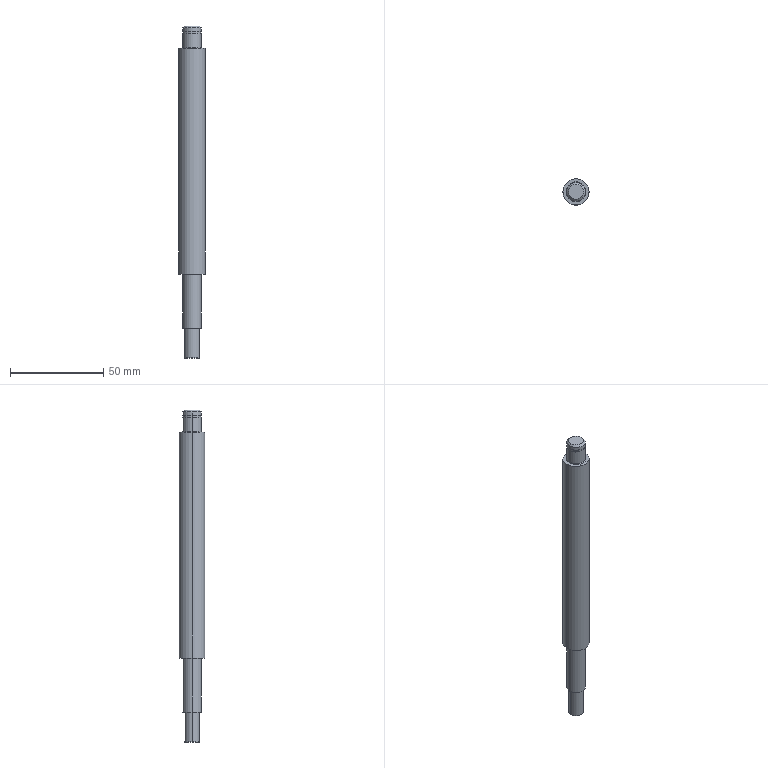Part | STEP file | 001-011-LHC07-D14-L178-S16 | 1 solid | 27 faces | box 14 x 14 x 178 mm | volume 22630 mm3 | cylinder 12 | plane 7 | cone 4 | torus 4 | commonest cylinder face diameters 10 x6 8 x2 9.6 x2 14 x2